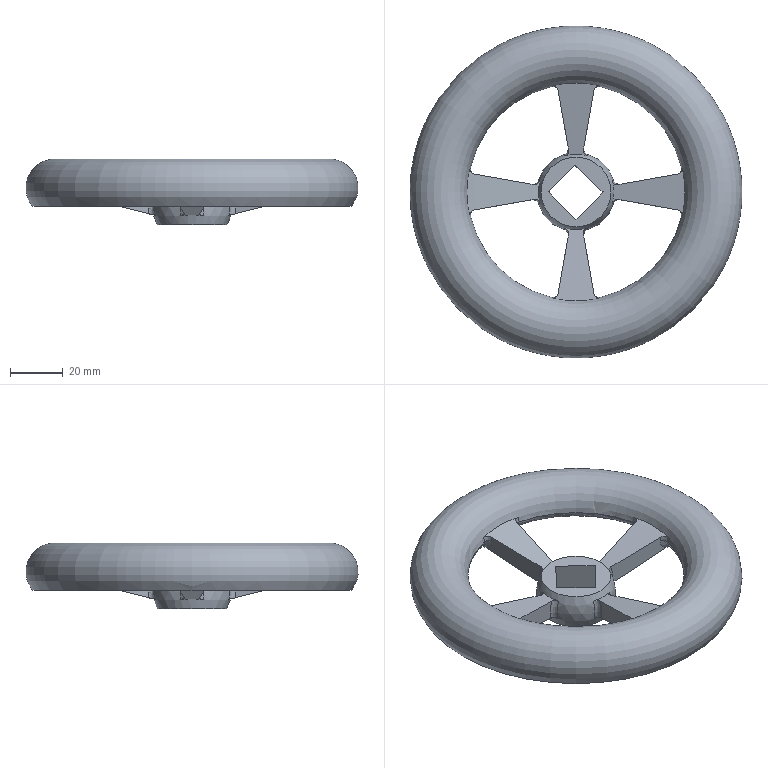Part | NX | features DATUM_CSYS 12, SKETCH 11, EXTRUDE 10, EXTRACT_DATUM_AXIS 8, EXTRACT_DATUM_PLANE 8, EXTRACT_FACE 8, EXTRACT_STRING 8, Instance Feature 6, BLEND 5, INTERSECT 4, Pattern Feature 2, UNITE 2, SPHERE 1, SWP104 1 | 1 solid | 56 faces | box 126 x 126 x 25 mm | volume 72074 mm3 | plane 23 | spline 16 | torus 12 | cylinder 4 | sphere 1 | commonest cylinder face diameters 87.847 x4